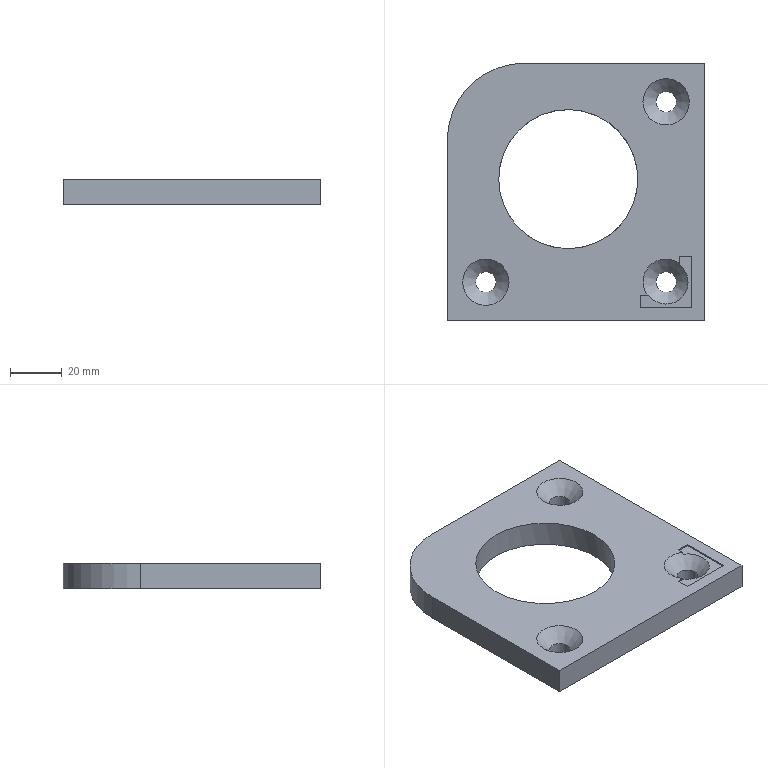Part | STEP file | solid 9 | 1 solid | 21 faces | box 100 x 100 x 10 mm | volume 72272 mm3 | plane 13 | cylinder 5 | cone 3 | commonest cylinder face diameters 8 x3 54 x1 60 x1